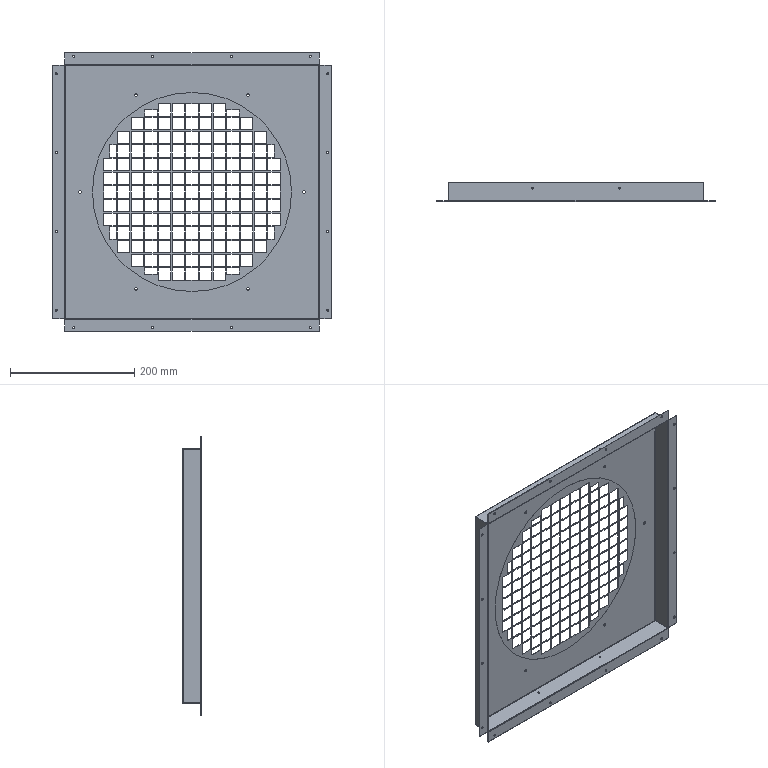Part | SolidWorks | features BaseBody 1 | 1 solid | 685 faces | box 448.8 x 29.9 x 448.6 mm | volume 111813 mm3 | plane 615 | cylinder 70 | commonest cylinder face diameters 3.5 x32 4.5 x12 0.4 x8 1.6 x8 2.5 x8 320 x2